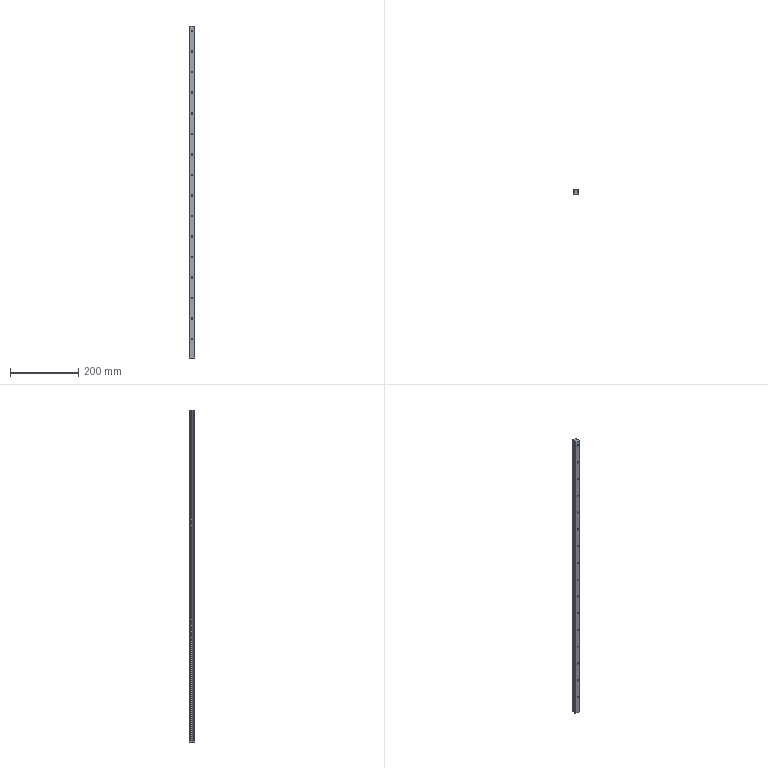Part | STEP file | HGR15-970 | 1 solid | 116 faces | box 15 x 15 x 970 mm | volume 178822 mm3 | cylinder 78 | plane 38 | commonest cylinder face diameters 4.5 x32 7.5 x32 0.8 x8 3.24 x4 2 x2